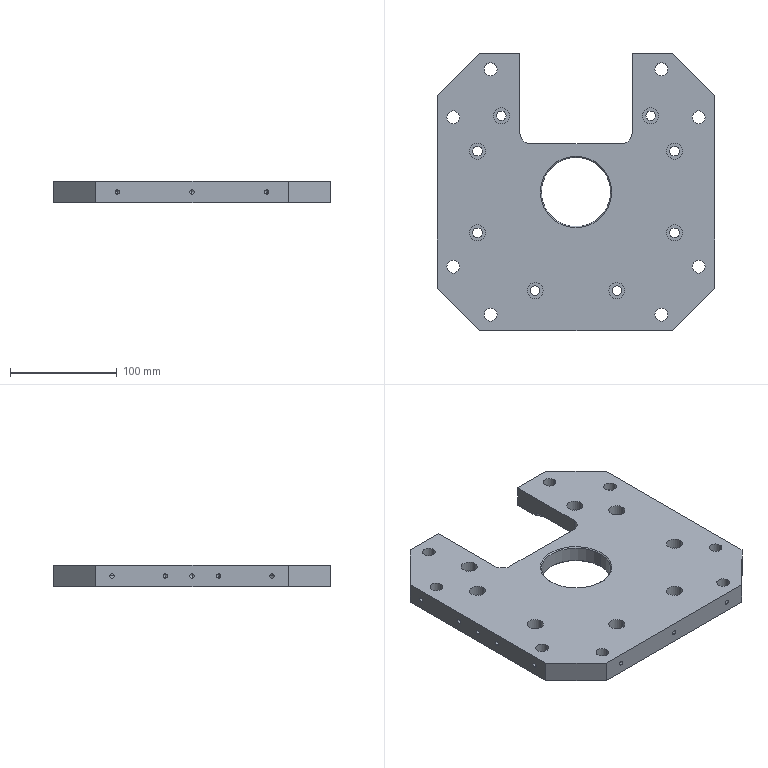Part | SolidWorks | features HoleWzd 6, Chamfer 3, ICE 2, Extrusion 1, Fillet 1 | 1 solid | 164 faces | box 260 x 260 x 20 mm | volume 876981 mm3 | cylinder 101 | plane 33 | cone 30 | commonest cylinder face diameters 4.2 x30 9 x16 12 x16 15 x16 18 x16 222.7 x3